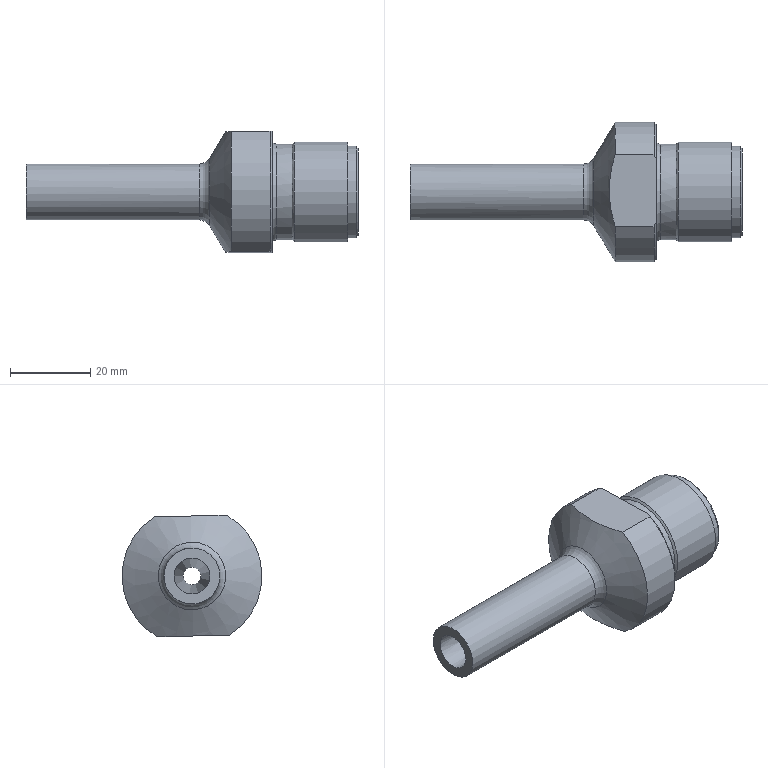Part | STEP file | 35-TOE-out(BIM35) | 1 solid | 24 faces | box 83 x 35 x 30.398 mm | volume 24144 mm3 | plane 7 | cone 7 | cylinder 7 | torus 3 | commonest cylinder face diameters 35 x2 14 x1 15 x1 23 x1 24 x1 25 x1